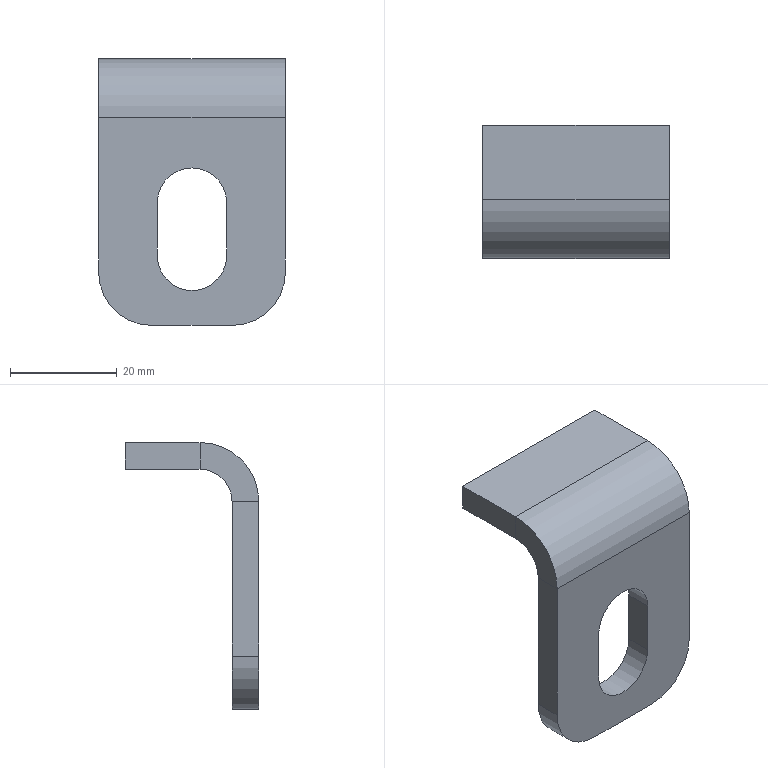Part | SolidWorks | features Fillet 1, FlatPattern 1, ICE 1, SMBaseFlange 1, SheetMetal 1, UnFold 1 | 1 solid | 21 faces | box 35 x 25 x 50 mm | volume 10083 mm3 | plane 14 | cylinder 7 | commonest cylinder face diameters 13 x3 20 x2 12 x1 22 x1
STEP:
#1=CARTESIAN_POINT('',(0.,0.,-20.5));
#2=VERTEX_POINT('',#1);
#3=CARTESIAN_POINT('',(6.5,0.,-27.));
#4=VERTEX_POINT('',#3);
#5=CARTESIAN_POINT('',(0.,0.,-27.));
#6=DIRECTION('',(0.,1.,0.));
#7=DIRECTION('',(0.,0.,1.));
#8=AXIS2_PLACEMENT_3D('',#5,#6,#7);
#9=CIRCLE('',#8,6.5);
#10=EDGE_CURVE('',#2,#4,#9,.T.);
#11=ORIENTED_EDGE('',*,*,#10,.F.);
#12=CARTESIAN_POINT('',(0.,5.,-20.5));
#13=VERTEX_POINT('',#12);
#14=CARTESIAN_POINT('',(0.,0.,-20.5));
#15=DIRECTION('',(0.,1.,0.));
#16=VECTOR('',#15,1000.);
#17=LINE('',#14,#16);
#18=EDGE_CURVE('',#2,#13,#17,.T.);
#19=ORIENTED_EDGE('',*,*,#18,.T.);
#20=CARTESIAN_POINT('',(6.5,5.,-27.));
#21=VERTEX_POINT('',#20);
#22=CARTESIAN_POINT('',(0.,5.,-27.));
#23=DIRECTION('',(0.,1.,0.));
#24=DIRECTION('',(0.,0.,1.));
#25=AXIS2_PLACEMENT_3D('',#22,#23,#24);
#26=CIRCLE('',#25,6.5);
#27=EDGE_CURVE('',#13,#21,#26,.T.);
#28=ORIENTED_EDGE('',*,*,#27,.T.);
#29=CARTESIAN_POINT('',(6.5,0.,-27.));
#30=DIRECTION('',(0.,1.,0.));
#31=VECTOR('',#30,1000.);
#32=LINE('',#29,#31);
#33=EDGE_CURVE('',#4,#21,#32,.T.);
#34=ORIENTED_EDGE('',*,*,#33,.F.);
#35=EDGE_LOOP('',(#11,#19,#28,#34));
#36=FACE_OUTER_BOUND('',#35,.T.);
#37=CARTESIAN_POINT('',(0.,0.,-27.));
#38=DIRECTION('',(0.,1.,0.));
#39=DIRECTION('',(0.,0.,1.));
#40=AXIS2_PLACEMENT_3D('',#37,#38,#39);
#41=CYLINDRICAL_SURFACE('',#40,6.5);
#42=ADVANCED_FACE('',(#36),#41,.F.);
#43=CARTESIAN_POINT('',(17.5,11.,0.));
#44=VERTEX_POINT('',#43);
#45=CARTESIAN_POINT('',(17.5,11.,-5.));
#46=VERTEX_POINT('',#45);
#47=CARTESIAN_POINT('',(17.5,11.,0.));
#48=DIRECTION('',(0.,0.,-1.));
#49=VECTOR('',#48,1000.);
#50=LINE('',#47,#49);
#51=EDGE_CURVE('',#44,#46,#50,.T.);
#52=ORIENTED_EDGE('',*,*,#51,.F.);
#53=CARTESIAN_POINT('',(17.5,0.,-11.));
#54=VERTEX_POINT('',#53);
#55=CARTESIAN_POINT('',(17.5,11.,-11.));
#56=DIRECTION('',(-1.,0.,0.));
#57=DIRECTION('',(0.,0.,-1.));
#58=AXIS2_PLACEMENT_3D('',#55,#56,#57);
#59=CIRCLE('',#58,11.);
#60=EDGE_CURVE('',#54,#44,#59,.T.);
#61=ORIENTED_EDGE('',*,*,#60,.F.);
#62=CARTESIAN_POINT('',(17.5,5.,-11.));
#63=VERTEX_POINT('',#62);
#64=CARTESIAN_POINT('',(17.5,5.,-11.));
#65=DIRECTION('',(0.,-1.,0.));
#66=VECTOR('',#65,1000.);
#67=LINE('',#64,#66);
#68=EDGE_CURVE('',#63,#54,#67,.T.);
#69=ORIENTED_EDGE('',*,*,#68,.F.);
#70=CARTESIAN_POINT('',(17.5,11.,-11.));
#71=DIRECTION('',(-1.,0.,0.));
#72=DIRECTION('',(0.,0.,-1.));
#73=AXIS2_PLACEMENT_3D('',#70,#71,#72);
#74=CIRCLE('',#73,6.);
#75=EDGE_CURVE('',#63,#46,#74,.T.);
#76=ORIENTED_EDGE('',*,*,#75,.T.);
#77=EDGE_LOOP('',(#52,#61,#69,#76));
#78=FACE_OUTER_BOUND('',#77,.T.);
#79=CARTESIAN_POINT('',(17.5,11.,0.));
#80=DIRECTION('',(1.,0.,0.));
#81=DIRECTION('',(0.,0.,-1.));
#82=AXIS2_PLACEMENT_3D('',#79,#80,#81);
#83=PLANE('',#82);
#84=ADVANCED_FACE('',(#78),#83,.T.);
#85=CARTESIAN_POINT('',(17.5,25.,0.));
#86=VERTEX_POINT('',#85);
#87=CARTESIAN_POINT('',(17.5,0.,0.));
#88=DIRECTION('',(0.,1.,0.));
#89=VECTOR('',#88,1000.);
#90=LINE('',#87,#89);
#91=EDGE_CURVE('',#44,#86,#90,.T.);
#92=ORIENTED_EDGE('',*,*,#91,.F.);
#93=ORIENTED_EDGE('',*,*,#51,.T.);
#94=CARTESIAN_POINT('',(17.5,25.,-5.));
#95=VERTEX_POINT('',#94);
#96=CARTESIAN_POINT('',(17.5,0.,-5.));
#97=DIRECTION('',(0.,1.,0.));
#98=VECTOR('',#97,1000.);
#99=LINE('',#96,#98);
#100=EDGE_CURVE('',#46,#95,#99,.T.);
#101=ORIENTED_EDGE('',*,*,#100,.T.);
#102=CARTESIAN_POINT('',(17.5,25.,0.));
#103=DIRECTION('',(0.,0.,-1.));
#104=VECTOR('',#103,1000.);
#105=LINE('',#102,#104);
#106=EDGE_CURVE('',#86,#95,#105,.T.);
#107=ORIENTED_EDGE('',*,*,#106,.F.);
#108=EDGE_LOOP('',(#92,#93,#101,#107));
#109=FACE_OUTER_BOUND('',#108,.T.);
#110=CARTESIAN_POINT('',(17.5,5.,-11.));
#111=DIRECTION('',(1.,0.,0.));
#112=DIRECTION('',(0.,0.,-1.));
#113=AXIS2_PLACEMENT_3D('',#110,#111,#112);
#114=PLANE('',#113);
#115=ADVANCED_FACE('',(#109),#114,.T.);
#116=CARTESIAN_POINT('',(-17.5,0.,-11.));
#117=VERTEX_POINT('',#116);
#118=CARTESIAN_POINT('',(-17.5,5.,-11.));
#119=VERTEX_POINT('',#118);
#120=CARTESIAN_POINT('',(-17.5,0.,-11.));
#121=DIRECTION('',(0.,1.,0.));
#122=VECTOR('',#121,1000.);
#123=LINE('',#120,#122);
#124=EDGE_CURVE('',#117,#119,#123,.T.);
#125=ORIENTED_EDGE('',*,*,#124,.F.);
#126=CARTESIAN_POINT('',(-17.5,11.,0.));
#127=VERTEX_POINT('',#126);
#128=CARTESIAN_POINT('',(-17.5,11.,-11.));
#129=DIRECTION('',(-1.,0.,0.));
#130=DIRECTION('',(0.,0.,-1.));
#131=AXIS2_PLACEMENT_3D('',#128,#129,#130);
#132=CIRCLE('',#131,11.);
#133=EDGE_CURVE('',#117,#127,#132,.T.);
#134=ORIENTED_EDGE('',*,*,#133,.T.);
#135=CARTESIAN_POINT('',(-17.5,11.,-5.));
#136=VERTEX_POINT('',#135);
#137=CARTESIAN_POINT('',(-17.5,11.,-5.));
#138=DIRECTION('',(0.,0.,1.));
#139=VECTOR('',#138,1000.);
#140=LINE('',#137,#139);
#141=EDGE_CURVE('',#136,#127,#140,.T.);
#142=ORIENTED_EDGE('',*,*,#141,.F.);
#143=CARTESIAN_POINT('',(-17.5,11.,-11.));
#144=DIRECTION('',(-1.,0.,0.));
#145=DIRECTION('',(0.,0.,-1.));
#146=AXIS2_PLACEMENT_3D('',#143,#144,#145);
#147=CIRCLE('',#146,6.);
#148=EDGE_CURVE('',#119,#136,#147,.T.);
#149=ORIENTED_EDGE('',*,*,#148,.F.);
#150=EDGE_LOOP('',(#125,#134,#142,#149));
#151=FACE_OUTER_BOUND('',#150,.T.);
#152=CARTESIAN_POINT('',(-17.5,0.,-11.));
#153=DIRECTION('',(-1.,0.,0.));
#154=DIRECTION('',(0.,0.,1.));
#155=AXIS2_PLACEMENT_3D('',#152,#153,#154);
#156=PLANE('',#155);
#157=ADVANCED_FACE('',(#151),#156,.T.);
#158=CARTESIAN_POINT('',(-17.5,5.,-40.));
#159=VERTEX_POINT('',#158);
#160=CARTESIAN_POINT('',(-17.5,5.,0.));
#161=DIRECTION('',(0.,0.,1.));
#162=VECTOR('',#161,1000.);
#163=LINE('',#160,#162);
#164=EDGE_CURVE('',#159,#119,#163,.T.);
#165=ORIENTED_EDGE('',*,*,#164,.F.);
#166=CARTESIAN_POINT('',(-17.5,0.,-40.));
#167=VERTEX_POINT('',#166);
#168=CARTESIAN_POINT('',(-17.5,11.,-40.));
#169=DIRECTION('',(0.,-1.,0.));
#170=VECTOR('',#169,1000.);
#171=LINE('',#168,#170);
#172=EDGE_CURVE('',#159,#167,#171,.T.);
#173=ORIENTED_EDGE('',*,*,#172,.T.);
#174=CARTESIAN_POINT('',(-17.5,0.,0.));
#175=DIRECTION('',(0.,0.,1.));
#176=VECTOR('',#175,1000.);
#177=LINE('',#174,#176);
#178=EDGE_CURVE('',#167,#117,#177,.T.);
#179=ORIENTED_EDGE('',*,*,#178,.T.);
#180=ORIENTED_EDGE('',*,*,#124,.T.);
#181=EDGE_LOOP('',(#165,#173,#179,#180));
#182=FACE_OUTER_BOUND('',#181,.T.);
#183=CARTESIAN_POINT('',(-17.5,11.,-5.));
#184=DIRECTION('',(-1.,0.,0.));
#185=DIRECTION('',(0.,0.,1.));
#186=AXIS2_PLACEMENT_3D('',#183,#184,#185);
#187=PLANE('',#186);
#188=ADVANCED_FACE('',(#182),#187,.T.);
#189=CARTESIAN_POINT('',(-17.5,25.,-5.));
#190=VERTEX_POINT('',#189);
#191=CARTESIAN_POINT('',(-17.5,0.,-5.));
#192=DIRECTION('',(0.,1.,0.));
#193=VECTOR('',#192,1000.);
#194=LINE('',#191,#193);
#195=EDGE_CURVE('',#136,#190,#194,.T.);
#196=ORIENTED_EDGE('',*,*,#195,.T.);
#197=CARTESIAN_POINT('',(17.5,25.,-5.));
#198=DIRECTION('',(-1.,0.,0.));
#199=VECTOR('',#198,1000.);
#200=LINE('',#197,#199);
#201=EDGE_CURVE('',#95,#190,#200,.T.);
#202=ORIENTED_EDGE('',*,*,#201,.F.);
#203=ORIENTED_EDGE('',*,*,#100,.F.);
#204=CARTESIAN_POINT('',(17.5,11.,-5.));
#205=DIRECTION('',(-1.,0.,0.));
#206=VECTOR('',#205,1000.);
#207=LINE('',#204,#206);
#208=EDGE_CURVE('',#46,#136,#207,.T.);
#209=ORIENTED_EDGE('',*,*,#208,.T.);
#210=EDGE_LOOP('',(#196,#202,#203,#209));
#211=FACE_OUTER_BOUND('',#210,.T.);
#212=CARTESIAN_POINT('',(17.5,0.,-5.));
#213=DIRECTION('',(0.,0.,1.));
#214=DIRECTION('',(1.,0.,0.));
#215=AXIS2_PLACEMENT_3D('',#212,#213,#214);
#216=PLANE('',#215);
#217=ADVANCED_FACE('',(#211),#216,.F.);
#218=CARTESIAN_POINT('',(-17.5,25.,0.));
#219=VERTEX_POINT('',#218);
#220=CARTESIAN_POINT('',(-17.5,25.,0.));
#221=DIRECTION('',(0.,0.,-1.));
#222=VECTOR('',#221,1000.);
#223=LINE('',#220,#222);
#224=EDGE_CURVE('',#219,#190,#223,.T.);
#225=ORIENTED_EDGE('',*,*,#224,.F.);
#226=CARTESIAN_POINT('',(17.5,25.,0.));
#227=DIRECTION('',(-1.,0.,0.));
#228=VECTOR('',#227,1000.);
#229=LINE('',#226,#228);
#230=EDGE_CURVE('',#86,#219,#229,.T.);
#231=ORIENTED_EDGE('',*,*,#230,.F.);
#232=ORIENTED_EDGE('',*,*,#106,.T.);
#233=ORIENTED_EDGE('',*,*,#201,.T.);
#234=EDGE_LOOP('',(#225,#231,#232,#233));
#235=FACE_OUTER_BOUND('',#234,.T.);
#236=CARTESIAN_POINT('',(17.5,25.,0.));
#237=DIRECTION('',(0.,1.,0.));
#238=DIRECTION('',(0.,0.,1.));
#239=AXIS2_PLACEMENT_3D('',#236,#237,#238);
#240=PLANE('',#239);
#241=ADVANCED_FACE('',(#235),#240,.T.);
#242=CARTESIAN_POINT('',(-17.5,0.,0.));
#243=DIRECTION('',(0.,1.,0.));
#244=VECTOR('',#243,1000.);
#245=LINE('',#242,#244);
#246=EDGE_CURVE('',#127,#219,#245,.T.);
#247=ORIENTED_EDGE('',*,*,#246,.F.);
#248=CARTESIAN_POINT('',(17.5,11.,0.));
#249=DIRECTION('',(-1.,0.,0.));
#250=VECTOR('',#249,1000.);
#251=LINE('',#248,#250);
#252=EDGE_CURVE('',#44,#127,#251,.T.);
#253=ORIENTED_EDGE('',*,*,#252,.F.);
#254=ORIENTED_EDGE('',*,*,#91,.T.);
#255=ORIENTED_EDGE('',*,*,#230,.T.);
#256=EDGE_LOOP('',(#247,#253,#254,#255));
#257=FACE_OUTER_BOUND('',#256,.T.);
#258=CARTESIAN_POINT('',(17.5,0.,0.));
#259=DIRECTION('',(0.,0.,1.));
#260=DIRECTION('',(1.,0.,0.));
#261=AXIS2_PLACEMENT_3D('',#258,#259,#260);
#262=PLANE('',#261);
#263=ADVANCED_FACE('',(#257),#262,.T.);
#264=ORIENTED_EDGE('',*,*,#133,.F.);
#265=CARTESIAN_POINT('',(17.5,0.,-11.));
#266=DIRECTION('',(-1.,0.,0.));
#267=VECTOR('',#266,1000.);
#268=LINE('',#265,#267);
#269=EDGE_CURVE('',#54,#117,#268,.T.);
#270=ORIENTED_EDGE('',*,*,#269,.F.);
#271=ORIENTED_EDGE('',*,*,#60,.T.);
#272=ORIENTED_EDGE('',*,*,#252,.T.);
#273=EDGE_LOOP('',(#264,#270,#271,#272));
#274=FACE_OUTER_BOUND('',#273,.T.);
#275=CARTESIAN_POINT('',(17.5,11.,-11.));
#276=DIRECTION('',(-1.,0.,0.));
#277=DIRECTION('',(0.,0.,1.));
#278=AXIS2_PLACEMENT_3D('',#275,#276,#277);
#279=CYLINDRICAL_SURFACE('',#278,11.);
#280=ADVANCED_FACE('',(#274),#279,.T.);
#281=CARTESIAN_POINT('',(-6.5,0.,-27.));
#282=VERTEX_POINT('',#281);
#283=CARTESIAN_POINT('',(0.,0.,-27.));
#284=DIRECTION('',(0.,1.,0.));
#285=DIRECTION('',(0.,0.,1.));
#286=AXIS2_PLACEMENT_3D('',#283,#284,#285);
#287=CIRCLE('',#286,6.5);
#288=EDGE_CURVE('',#282,#2,#287,.T.);
#289=ORIENTED_EDGE('',*,*,#288,.T.);
#290=ORIENTED_EDGE('',*,*,#10,.T.);
#291=CARTESIAN_POINT('',(6.5,0.,-37.));
#292=VERTEX_POINT('',#291);
#293=CARTESIAN_POINT('',(6.5,0.,-27.));
#294=DIRECTION('',(0.,0.,-1.));
#295=VECTOR('',#294,1000.);
#296=LINE('',#293,#295);
#297=EDGE_CURVE('',#4,#292,#296,.T.);
#298=ORIENTED_EDGE('',*,*,#297,.T.);
#299=CARTESIAN_POINT('',(-6.5,0.,-37.));
#300=VERTEX_POINT('',#299);
#301=CARTESIAN_POINT('',(0.,0.,-37.));
#302=DIRECTION('',(0.,1.,0.));
#303=DIRECTION('',(0.,0.,1.));
#304=AXIS2_PLACEMENT_3D('',#301,#302,#303);
#305=CIRCLE('',#304,6.5);
#306=EDGE_CURVE('',#292,#300,#305,.T.);
#307=ORIENTED_EDGE('',*,*,#306,.T.);
#308=CARTESIAN_POINT('',(-6.5,0.,-27.));
#309=DIRECTION('',(0.,0.,1.));
#310=VECTOR('',#309,1000.);
#311=LINE('',#308,#310);
#312=EDGE_CURVE('',#300,#282,#311,.T.);
#313=ORIENTED_EDGE('',*,*,#312,.T.);
#314=EDGE_LOOP('',(#289,#290,#298,#307,#313));
#315=FACE_BOUND('',#314,.T.);
#316=ORIENTED_EDGE('',*,*,#178,.F.);
#317=CARTESIAN_POINT('',(-7.5,0.,-50.));
#318=VERTEX_POINT('',#317);
#319=CARTESIAN_POINT('',(-7.5,0.,-40.));
#320=DIRECTION('',(0.,-1.,0.));
#321=DIRECTION('',(0.,0.,-1.));
#322=AXIS2_PLACEMENT_3D('',#319,#320,#321);
#323=CIRCLE('',#322,10.);
#324=EDGE_CURVE('',#167,#318,#323,.T.);
#325=ORIENTED_EDGE('',*,*,#324,.T.);
#326=CARTESIAN_POINT('',(7.5,0.,-50.));
#327=VERTEX_POINT('',#326);
#328=CARTESIAN_POINT('',(17.5,0.,-50.));
#329=DIRECTION('',(-1.,0.,0.));
#330=VECTOR('',#329,1000.);
#331=LINE('',#328,#330);
#332=EDGE_CURVE('',#327,#318,#331,.T.);
#333=ORIENTED_EDGE('',*,*,#332,.F.);
#334=CARTESIAN_POINT('',(17.5,0.,-40.));
#335=VERTEX_POINT('',#334);
#336=CARTESIAN_POINT('',(7.5,0.,-40.));
#337=DIRECTION('',(0.,-1.,0.));
#338=DIRECTION('',(0.,0.,-1.));
#339=AXIS2_PLACEMENT_3D('',#336,#337,#338);
#340=CIRCLE('',#339,10.);
#341=EDGE_CURVE('',#327,#335,#340,.T.);
#342=ORIENTED_EDGE('',*,*,#341,.T.);
#343=CARTESIAN_POINT('',(17.5,0.,0.));
#344=DIRECTION('',(0.,0.,1.));
#345=VECTOR('',#344,1000.);
#346=LINE('',#343,#345);
#347=EDGE_CURVE('',#335,#54,#346,.T.);
#348=ORIENTED_EDGE('',*,*,#347,.T.);
#349=ORIENTED_EDGE('',*,*,#269,.T.);
#350=EDGE_LOOP('',(#316,#325,#333,#342,#348,#349));
#351=FACE_OUTER_BOUND('',#350,.T.);
#352=CARTESIAN_POINT('',(17.5,0.,0.));
#353=DIRECTION('',(0.,-1.,0.));
#354=DIRECTION('',(0.,0.,-1.));
#355=AXIS2_PLACEMENT_3D('',#352,#353,#354);
#356=PLANE('',#355);
#357=ADVANCED_FACE('',(#315,#351),#356,.T.);
#358=ORIENTED_EDGE('',*,*,#332,.T.);
#359=CARTESIAN_POINT('',(-7.5,5.,-50.));
#360=VERTEX_POINT('',#359);
#361=CARTESIAN_POINT('',(-7.5,5.,-50.));
#362=DIRECTION('',(0.,1.,0.));
#363=VECTOR('',#362,1000.);
#364=LINE('',#361,#363);
#365=EDGE_CURVE('',#318,#360,#364,.T.);
#366=ORIENTED_EDGE('',*,*,#365,.T.);
#367=CARTESIAN_POINT('',(7.5,5.,-50.));
#368=VERTEX_POINT('',#367);
#369=CARTESIAN_POINT('',(17.5,5.,-50.));
#370=DIRECTION('',(-1.,0.,0.));
#371=VECTOR('',#370,1000.);
#372=LINE('',#369,#371);
#373=EDGE_CURVE('',#368,#360,#372,.T.);
#374=ORIENTED_EDGE('',*,*,#373,.F.);
#375=CARTESIAN_POINT('',(7.5,5.,-50.));
#376=DIRECTION('',(0.,-1.,0.));
#377=VECTOR('',#376,1000.);
#378=LINE('',#375,#377);
#379=EDGE_CURVE('',#368,#327,#378,.T.);
#380=ORIENTED_EDGE('',*,*,#379,.T.);
#381=EDGE_LOOP('',(#358,#366,#374,#380));
#382=FACE_OUTER_BOUND('',#381,.T.);
#383=CARTESIAN_POINT('',(17.5,5.,-50.));
#384=DIRECTION('',(0.,0.,-1.));
#385=DIRECTION('',(-1.,0.,0.));
#386=AXIS2_PLACEMENT_3D('',#383,#384,#385);
#387=PLANE('',#386);
#388=ADVANCED_FACE('',(#382),#387,.T.);
#389=CARTESIAN_POINT('',(6.5,5.,-37.));
#390=VERTEX_POINT('',#389);
#391=CARTESIAN_POINT('',(6.5,5.,-27.));
#392=DIRECTION('',(0.,0.,-1.));
#393=VECTOR('',#392,1000.);
#394=LINE('',#391,#393);
#395=EDGE_CURVE('',#21,#390,#394,.T.);
#396=ORIENTED_EDGE('',*,*,#395,.F.);
#397=ORIENTED_EDGE('',*,*,#27,.F.);
#398=CARTESIAN_POINT('',(-6.5,5.,-27.));
#399=VERTEX_POINT('',#398);
#400=CARTESIAN_POINT('',(0.,5.,-27.));
#401=DIRECTION('',(0.,1.,0.));
#402=DIRECTION('',(0.,0.,1.));
#403=AXIS2_PLACEMENT_3D('',#400,#401,#402);
#404=CIRCLE('',#403,6.5);
#405=EDGE_CURVE('',#399,#13,#404,.T.);
#406=ORIENTED_EDGE('',*,*,#405,.F.);
#407=CARTESIAN_POINT('',(-6.5,5.,-37.));
#408=VERTEX_POINT('',#407);
#409=CARTESIAN_POINT('',(-6.5,5.,-27.));
#410=DIRECTION('',(0.,0.,1.));
#411=VECTOR('',#410,1000.);
#412=LINE('',#409,#411);
#413=EDGE_CURVE('',#408,#399,#412,.T.);
#414=ORIENTED_EDGE('',*,*,#413,.F.);
#415=CARTESIAN_POINT('',(0.,5.,-37.));
#416=DIRECTION('',(0.,1.,0.));
#417=DIRECTION('',(0.,0.,1.));
#418=AXIS2_PLACEMENT_3D('',#415,#416,#417);
#419=CIRCLE('',#418,6.5);
#420=EDGE_CURVE('',#390,#408,#419,.T.);
#421=ORIENTED_EDGE('',*,*,#420,.F.);
#422=EDGE_LOOP('',(#396,#397,#406,#414,#421));
#423=FACE_BOUND('',#422,.T.);
#424=ORIENTED_EDGE('',*,*,#373,.T.);
#425=CARTESIAN_POINT('',(-7.5,5.,-40.));
#426=DIRECTION('',(0.,1.,0.));
#427=DIRECTION('',(0.,0.,-1.));
#428=AXIS2_PLACEMENT_3D('',#425,#426,#427);
#429=CIRCLE('',#428,10.);
#430=EDGE_CURVE('',#360,#159,#429,.T.);
#431=ORIENTED_EDGE('',*,*,#430,.T.);
#432=ORIENTED_EDGE('',*,*,#164,.T.);
#433=CARTESIAN_POINT('',(17.5,5.,-11.));
#434=DIRECTION('',(-1.,0.,0.));
#435=VECTOR('',#434,1000.);
#436=LINE('',#433,#435);
#437=EDGE_CURVE('',#63,#119,#436,.T.);
#438=ORIENTED_EDGE('',*,*,#437,.F.);
#439=CARTESIAN_POINT('',(17.5,5.,-40.));
#440=VERTEX_POINT('',#439);
#441=CARTESIAN_POINT('',(17.5,5.,0.));
#442=DIRECTION('',(0.,0.,1.));
#443=VECTOR('',#442,1000.);
#444=LINE('',#441,#443);
#445=EDGE_CURVE('',#440,#63,#444,.T.);
#446=ORIENTED_EDGE('',*,*,#445,.F.);
#447=CARTESIAN_POINT('',(7.5,5.,-40.));
#448=DIRECTION('',(0.,1.,0.));
#449=DIRECTION('',(0.,0.,-1.));
#450=AXIS2_PLACEMENT_3D('',#447,#448,#449);
#451=CIRCLE('',#450,10.);
#452=EDGE_CURVE('',#440,#368,#451,.T.);
#453=ORIENTED_EDGE('',*,*,#452,.T.);
#454=EDGE_LOOP('',(#424,#431,#432,#438,#446,#453));
#455=FACE_OUTER_BOUND('',#454,.T.);
#456=CARTESIAN_POINT('',(17.5,5.,0.));
#457=DIRECTION('',(0.,-1.,0.));
#458=DIRECTION('',(0.,0.,-1.));
#459=AXIS2_PLACEMENT_3D('',#456,#457,#458);
#460=PLANE('',#459);
#461=ADVANCED_FACE('',(#423,#455),#460,.F.);
#462=ORIENTED_EDGE('',*,*,#148,.T.);
#463=ORIENTED_EDGE('',*,*,#208,.F.);
#464=ORIENTED_EDGE('',*,*,#75,.F.);
#465=ORIENTED_EDGE('',*,*,#437,.T.);
#466=EDGE_LOOP('',(#462,#463,#464,#465));
#467=FACE_OUTER_BOUND('',#466,.T.);
#468=CARTESIAN_POINT('',(17.5,11.,-11.));
#469=DIRECTION('',(-1.,0.,0.));
#470=DIRECTION('',(0.,0.,1.));
#471=AXIS2_PLACEMENT_3D('',#468,#469,#470);
#472=CYLINDRICAL_SURFACE('',#471,6.);
#473=ADVANCED_FACE('',(#467),#472,.F.);
#474=ORIENTED_EDGE('',*,*,#347,.F.);
#475=CARTESIAN_POINT('',(17.5,11.,-40.));
#476=DIRECTION('',(0.,1.,0.));
#477=VECTOR('',#476,1000.);
#478=LINE('',#475,#477);
#479=EDGE_CURVE('',#335,#440,#478,.T.);
#480=ORIENTED_EDGE('',*,*,#479,.T.);
#481=ORIENTED_EDGE('',*,*,#445,.T.);
#482=ORIENTED_EDGE('',*,*,#68,.T.);
#483=EDGE_LOOP('',(#474,#480,#481,#482));
#484=FACE_OUTER_BOUND('',#483,.T.);
#485=CARTESIAN_POINT('',(17.5,11.,-11.));
#486=DIRECTION('',(1.,0.,0.));
#487=DIRECTION('',(0.,0.,-1.));
#488=AXIS2_PLACEMENT_3D('',#485,#486,#487);
#489=PLANE('',#488);
#490=ADVANCED_FACE('',(#484),#489,.T.);
#491=ORIENTED_EDGE('',*,*,#195,.F.);
#492=ORIENTED_EDGE('',*,*,#141,.T.);
#493=ORIENTED_EDGE('',*,*,#246,.T.);
#494=ORIENTED_EDGE('',*,*,#224,.T.);
#495=EDGE_LOOP('',(#491,#492,#493,#494));
#496=FACE_OUTER_BOUND('',#495,.T.);
#497=CARTESIAN_POINT('',(-17.5,11.,-11.));
#498=DIRECTION('',(1.,0.,0.));
#499=DIRECTION('',(0.,0.,-1.));
#500=AXIS2_PLACEMENT_3D('',#497,#498,#499);
#501=PLANE('',#500);
#502=ADVANCED_FACE('',(#496),#501,.F.);
#503=ORIENTED_EDGE('',*,*,#18,.F.);
#504=ORIENTED_EDGE('',*,*,#288,.F.);
#505=CARTESIAN_POINT('',(-6.5,0.,-27.));
#506=DIRECTION('',(0.,1.,0.));
#507=VECTOR('',#506,1000.);
#508=LINE('',#505,#507);
#509=EDGE_CURVE('',#282,#399,#508,.T.);
#510=ORIENTED_EDGE('',*,*,#509,.T.);
#511=ORIENTED_EDGE('',*,*,#405,.T.);
#512=EDGE_LOOP('',(#503,#504,#510,#511));
#513=FACE_OUTER_BOUND('',#512,.T.);
#514=CARTESIAN_POINT('',(0.,0.,-27.));
#515=DIRECTION('',(0.,1.,0.));
#516=DIRECTION('',(0.,0.,1.));
#517=AXIS2_PLACEMENT_3D('',#514,#515,#516);
#518=CYLINDRICAL_SURFACE('',#517,6.5);
#519=ADVANCED_FACE('',(#513),#518,.F.);
#520=ORIENTED_EDGE('',*,*,#413,.T.);
#521=ORIENTED_EDGE('',*,*,#509,.F.);
#522=ORIENTED_EDGE('',*,*,#312,.F.);
#523=CARTESIAN_POINT('',(-6.5,0.,-37.));
#524=DIRECTION('',(0.,1.,0.));
#525=VECTOR('',#524,1000.);
#526=LINE('',#523,#525);
#527=EDGE_CURVE('',#300,#408,#526,.T.);
#528=ORIENTED_EDGE('',*,*,#527,.T.);
#529=EDGE_LOOP('',(#520,#521,#522,#528));
#530=FACE_OUTER_BOUND('',#529,.T.);
#531=CARTESIAN_POINT('',(-6.5,0.,-27.));
#532=DIRECTION('',(-1.,0.,0.));
#533=DIRECTION('',(0.,0.,1.));
#534=AXIS2_PLACEMENT_3D('',#531,#532,#533);
#535=PLANE('',#534);
#536=ADVANCED_FACE('',(#530),#535,.F.);
#537=ORIENTED_EDGE('',*,*,#420,.T.);
#538=ORIENTED_EDGE('',*,*,#527,.F.);
#539=ORIENTED_EDGE('',*,*,#306,.F.);
#540=CARTESIAN_POINT('',(6.5,0.,-37.));
#541=DIRECTION('',(0.,1.,0.));
#542=VECTOR('',#541,1000.);
#543=LINE('',#540,#542);
#544=EDGE_CURVE('',#292,#390,#543,.T.);
#545=ORIENTED_EDGE('',*,*,#544,.T.);
#546=EDGE_LOOP('',(#537,#538,#539,#545));
#547=FACE_OUTER_BOUND('',#546,.T.);
#548=CARTESIAN_POINT('',(0.,0.,-37.));
#549=DIRECTION('',(0.,1.,0.));
#550=DIRECTION('',(0.,0.,1.));
#551=AXIS2_PLACEMENT_3D('',#548,#549,#550);
#552=CYLINDRICAL_SURFACE('',#551,6.5);
#553=ADVANCED_FACE('',(#547),#552,.F.);
#554=ORIENTED_EDGE('',*,*,#395,.T.);
#555=ORIENTED_EDGE('',*,*,#544,.F.);
#556=ORIENTED_EDGE('',*,*,#297,.F.);
#557=ORIENTED_EDGE('',*,*,#33,.T.);
#558=EDGE_LOOP('',(#554,#555,#556,#557));
#559=FACE_OUTER_BOUND('',#558,.T.);
#560=CARTESIAN_POINT('',(6.5,0.,-27.));
#561=DIRECTION('',(1.,0.,0.));
#562=DIRECTION('',(0.,0.,-1.));
#563=AXIS2_PLACEMENT_3D('',#560,#561,#562);
#564=PLANE('',#563);
#565=ADVANCED_FACE('',(#559),#564,.F.);
#566=ORIENTED_EDGE('',*,*,#430,.F.);
#567=ORIENTED_EDGE('',*,*,#365,.F.);
#568=ORIENTED_EDGE('',*,*,#324,.F.);
#569=ORIENTED_EDGE('',*,*,#172,.F.);
#570=EDGE_LOOP('',(#566,#567,#568,#569));
#571=FACE_OUTER_BOUND('',#570,.T.);
#572=CARTESIAN_POINT('',(-7.5,11.,-40.));
#573=DIRECTION('',(0.,-1.,0.));
#574=DIRECTION('',(0.,0.,-1.));
#575=AXIS2_PLACEMENT_3D('',#572,#573,#574);
#576=CYLINDRICAL_SURFACE('',#575,10.);
#577=ADVANCED_FACE('',(#571),#576,.T.);
#578=ORIENTED_EDGE('',*,*,#452,.F.);
#579=ORIENTED_EDGE('',*,*,#479,.F.);
#580=ORIENTED_EDGE('',*,*,#341,.F.);
#581=ORIENTED_EDGE('',*,*,#379,.F.);
#582=EDGE_LOOP('',(#578,#579,#580,#581));
#583=FACE_OUTER_BOUND('',#582,.T.);
#584=CARTESIAN_POINT('',(7.5,5.,-40.));
#585=DIRECTION('',(0.,-1.,0.));
#586=DIRECTION('',(0.,0.,-1.));
#587=AXIS2_PLACEMENT_3D('',#584,#585,#586);
#588=CYLINDRICAL_SURFACE('',#587,10.);
#589=ADVANCED_FACE('',(#583),#588,.T.);
#590=CLOSED_SHELL('',(#42,#84,#115,#157,#188,#217,#241,#263,#280,#357,#388,#461,#473,#490,#502,#519,#536,#553,#565,#577,#589));
#591=MANIFOLD_SOLID_BREP('',#590);
#592=CARTESIAN_POINT('',(0.,0.,0.));
#593=DIRECTION('',(0.,0.,1.));
#594=DIRECTION('',(1.,0.,0.));
#595=AXIS2_PLACEMENT_3D('',#592,#593,#594);
#596=(LENGTH_UNIT()NAMED_UNIT(*)SI_UNIT(.MILLI.,.METRE.));
#597=UNCERTAINTY_MEASURE_WITH_UNIT(LENGTH_MEASURE(0.00001),#596,'','');
#598=(NAMED_UNIT(*)PLANE_ANGLE_UNIT()SI_UNIT($,.RADIAN.));
#599=(NAMED_UNIT(*)SI_UNIT($,.STERADIAN.)SOLID_ANGLE_UNIT());
#600=(GEOMETRIC_REPRESENTATION_CONTEXT(3)GLOBAL_UNCERTAINTY_ASSIGNED_CONTEXT((#597))GLOBAL_UNIT_ASSIGNED_CONTEXT((#596,#598,#599))REPRESENTATION_CONTEXT('',''));
#601=ADVANCED_BREP_SHAPE_REPRESENTATION('',(#591,#595),#600);